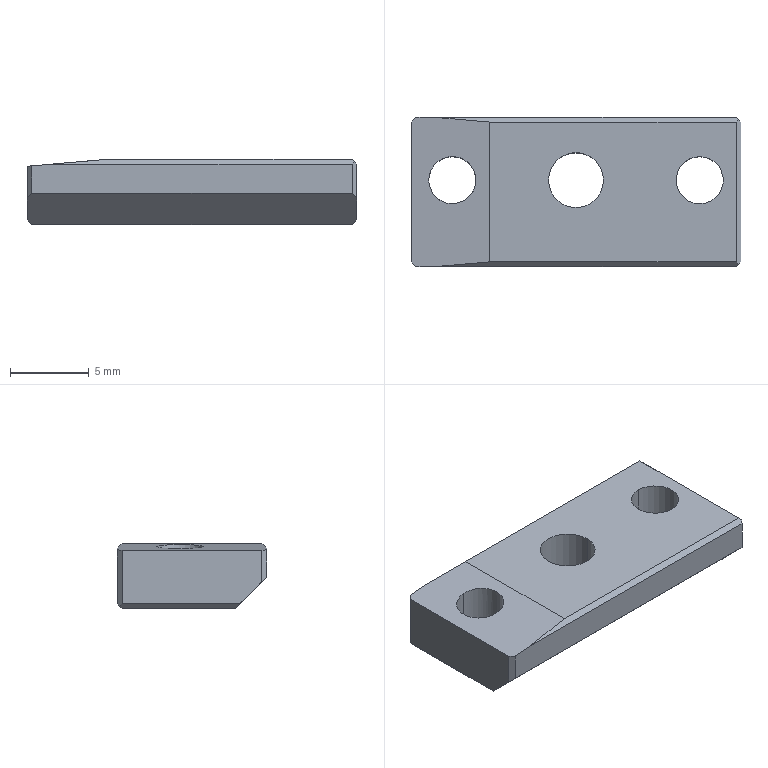Part | NX | 1 solid | 24 faces | box 21 x 9.5 x 4.15 mm | volume 674.351 mm3 | plane 18 | cylinder 6 | commonest cylinder face diameters 3 x4 3.5 x2
STEP:
#1=CARTESIAN_POINT('',(-137.,182.4,-96.5));
#2=VERTEX_POINT('',#1);
#3=CARTESIAN_POINT('',(-137.,173.5,-96.5));
#4=VERTEX_POINT('',#3);
#5=CARTESIAN_POINT('',(-137.,177.95,-96.5));
#6=DIRECTION('',(0.,-1.,0.));
#7=VECTOR('',#6,1000.);
#8=LINE('',#5,#7);
#9=EDGE_CURVE('',#2,#4,#8,.T.);
#10=ORIENTED_EDGE('',*,*,#9,.T.);
#11=CARTESIAN_POINT('',(-121.3,173.5,-96.5));
#12=VERTEX_POINT('',#11);
#13=CARTESIAN_POINT('',(-131.65,173.5,-96.5));
#14=DIRECTION('',(1.,0.,0.));
#15=VECTOR('',#14,1000.);
#16=LINE('',#13,#15);
#17=EDGE_CURVE('',#4,#12,#16,.T.);
#18=ORIENTED_EDGE('',*,*,#17,.T.);
#19=CARTESIAN_POINT('',(-121.3,182.4,-96.5));
#20=VERTEX_POINT('',#19);
#21=CARTESIAN_POINT('',(-121.3,177.95,-96.5));
#22=DIRECTION('',(0.,-1.,0.));
#23=VECTOR('',#22,1000.);
#24=LINE('',#21,#23);
#25=EDGE_CURVE('',#20,#12,#24,.T.);
#26=ORIENTED_EDGE('',*,*,#25,.F.);
#27=CARTESIAN_POINT('',(-131.65,182.4,-96.5));
#28=DIRECTION('',(-1.,0.,0.));
#29=VECTOR('',#28,1000.);
#30=LINE('',#27,#29);
#31=EDGE_CURVE('',#20,#2,#30,.T.);
#32=ORIENTED_EDGE('',*,*,#31,.T.);
#33=EDGE_LOOP('',(#10,#18,#26,#32));
#34=FACE_BOUND('',#33,.T.);
#35=CARTESIAN_POINT('',(-123.625,180.2,-96.5));
#36=VERTEX_POINT('',#35);
#37=CARTESIAN_POINT('',(-123.625,177.2,-96.5));
#38=VERTEX_POINT('',#37);
#39=CARTESIAN_POINT('',(-123.625,178.7,-96.5));
#40=DIRECTION('',(0.,0.,-1.));
#41=DIRECTION('',(0.,-1.,0.));
#42=AXIS2_PLACEMENT_3D('',#39,#40,#41);
#43=CIRCLE('',#42,1.5);
#44=EDGE_CURVE('',#36,#38,#43,.T.);
#45=ORIENTED_EDGE('',*,*,#44,.T.);
#46=CARTESIAN_POINT('',(-123.625,178.7,-96.5));
#47=DIRECTION('',(0.,0.,-1.));
#48=DIRECTION('',(0.,-1.,0.));
#49=AXIS2_PLACEMENT_3D('',#46,#47,#48);
#50=CIRCLE('',#49,1.5);
#51=EDGE_CURVE('',#38,#36,#50,.T.);
#52=ORIENTED_EDGE('',*,*,#51,.T.);
#53=EDGE_LOOP('',(#45,#52));
#54=FACE_BOUND('',#53,.T.);
#55=CARTESIAN_POINT('',(-129.75,178.7,-96.5));
#56=VERTEX_POINT('',#55);
#57=CARTESIAN_POINT('',(-133.25,178.7,-96.5));
#58=VERTEX_POINT('',#57);
#59=CARTESIAN_POINT('',(-131.5,178.7,-96.5));
#60=DIRECTION('',(0.,0.,-1.));
#61=DIRECTION('',(-1.,0.,0.));
#62=AXIS2_PLACEMENT_3D('',#59,#60,#61);
#63=CIRCLE('',#62,1.75);
#64=EDGE_CURVE('',#56,#58,#63,.T.);
#65=ORIENTED_EDGE('',*,*,#64,.T.);
#66=CARTESIAN_POINT('',(-131.5,178.7,-96.5));
#67=DIRECTION('',(0.,0.,-1.));
#68=DIRECTION('',(-1.,0.,0.));
#69=AXIS2_PLACEMENT_3D('',#66,#67,#68);
#70=CIRCLE('',#69,1.75);
#71=EDGE_CURVE('',#58,#56,#70,.T.);
#72=ORIENTED_EDGE('',*,*,#71,.T.);
#73=EDGE_LOOP('',(#65,#72));
#74=FACE_BOUND('',#73,.T.);
#75=CARTESIAN_POINT('',(-121.,182.7,-96.5));
#76=DIRECTION('',(0.,0.,1.));
#77=DIRECTION('',(1.,0.,0.));
#78=AXIS2_PLACEMENT_3D('',#75,#76,#77);
#79=PLANE('',#78);
#80=ADVANCED_FACE('',(#34,#54,#74),#79,.T.);
#81=CARTESIAN_POINT('',(-121.3,182.7,-96.8));
#82=VERTEX_POINT('',#81);
#83=CARTESIAN_POINT('',(-140.429,182.7,-96.8));
#84=VERTEX_POINT('',#83);
#85=CARTESIAN_POINT('',(-131.65,182.7,-96.8));
#86=DIRECTION('',(-1.,0.,0.));
#87=VECTOR('',#86,1000.);
#88=LINE('',#85,#87);
#89=EDGE_CURVE('',#82,#84,#88,.T.);
#90=ORIENTED_EDGE('',*,*,#89,.F.);
#91=CARTESIAN_POINT('',(-121.3,182.7,-100.35));
#92=VERTEX_POINT('',#91);
#93=CARTESIAN_POINT('',(-121.3,182.7,-98.575));
#94=DIRECTION('',(0.,0.,1.));
#95=VECTOR('',#94,1000.);
#96=LINE('',#93,#95);
#97=EDGE_CURVE('',#92,#82,#96,.T.);
#98=ORIENTED_EDGE('',*,*,#97,.F.);
#99=CARTESIAN_POINT('',(-141.7,182.7,-100.35));
#100=VERTEX_POINT('',#99);
#101=CARTESIAN_POINT('',(-131.5,182.7,-100.35));
#102=DIRECTION('',(-1.,0.,0.));
#103=VECTOR('',#102,1000.);
#104=LINE('',#101,#103);
#105=EDGE_CURVE('',#92,#100,#104,.T.);
#106=ORIENTED_EDGE('',*,*,#105,.T.);
#107=CARTESIAN_POINT('',(-141.7,182.7,-96.911));
#108=VERTEX_POINT('',#107);
#109=CARTESIAN_POINT('',(-141.7,182.7,-98.425));
#110=DIRECTION('',(0.,0.,1.));
#111=VECTOR('',#110,1000.);
#112=LINE('',#109,#111);
#113=EDGE_CURVE('',#100,#108,#112,.T.);
#114=ORIENTED_EDGE('',*,*,#113,.T.);
#115=CARTESIAN_POINT('',(-121.,182.7,-95.1));
#116=DIRECTION('',(-0.9962,0.,-0.08716));
#117=VECTOR('',#116,1000.);
#118=LINE('',#115,#117);
#119=EDGE_CURVE('',#84,#108,#118,.T.);
#120=ORIENTED_EDGE('',*,*,#119,.F.);
#121=EDGE_LOOP('',(#90,#98,#106,#114,#120));
#122=FACE_BOUND('',#121,.T.);
#123=CARTESIAN_POINT('',(-121.,182.7,-100.65));
#124=DIRECTION('',(0.,1.,0.));
#125=DIRECTION('',(1.,0.,0.));
#126=AXIS2_PLACEMENT_3D('',#123,#124,#125);
#127=PLANE('',#126);
#128=ADVANCED_FACE('',(#122),#127,.T.);
#129=CARTESIAN_POINT('',(-121.3,175.2,-100.65));
#130=VERTEX_POINT('',#129);
#131=CARTESIAN_POINT('',(-141.7,175.2,-100.65));
#132=VERTEX_POINT('',#131);
#133=CARTESIAN_POINT('',(-131.5,175.2,-100.65));
#134=DIRECTION('',(-1.,0.,0.));
#135=VECTOR('',#134,1000.);
#136=LINE('',#133,#135);
#137=EDGE_CURVE('',#130,#132,#136,.T.);
#138=ORIENTED_EDGE('',*,*,#137,.T.);
#139=CARTESIAN_POINT('',(-141.7,182.4,-100.65));
#140=VERTEX_POINT('',#139);
#141=CARTESIAN_POINT('',(-141.7,178.95,-100.65));
#142=DIRECTION('',(0.,1.,0.));
#143=VECTOR('',#142,1000.);
#144=LINE('',#141,#143);
#145=EDGE_CURVE('',#132,#140,#144,.T.);
#146=ORIENTED_EDGE('',*,*,#145,.T.);
#147=CARTESIAN_POINT('',(-121.3,182.4,-100.65));
#148=VERTEX_POINT('',#147);
#149=CARTESIAN_POINT('',(-131.5,182.4,-100.65));
#150=DIRECTION('',(-1.,0.,0.));
#151=VECTOR('',#150,1000.);
#152=LINE('',#149,#151);
#153=EDGE_CURVE('',#148,#140,#152,.T.);
#154=ORIENTED_EDGE('',*,*,#153,.F.);
#155=CARTESIAN_POINT('',(-121.3,178.95,-100.65));
#156=DIRECTION('',(0.,1.,0.));
#157=VECTOR('',#156,1000.);
#158=LINE('',#155,#157);
#159=EDGE_CURVE('',#130,#148,#158,.T.);
#160=ORIENTED_EDGE('',*,*,#159,.F.);
#161=EDGE_LOOP('',(#138,#146,#154,#160));
#162=FACE_BOUND('',#161,.T.);
#163=CARTESIAN_POINT('',(-129.75,178.7,-100.65));
#164=VERTEX_POINT('',#163);
#165=CARTESIAN_POINT('',(-133.25,178.7,-100.65));
#166=VERTEX_POINT('',#165);
#167=CARTESIAN_POINT('',(-131.5,178.7,-100.65));
#168=DIRECTION('',(0.,0.,-1.));
#169=DIRECTION('',(-1.,0.,0.));
#170=AXIS2_PLACEMENT_3D('',#167,#168,#169);
#171=CIRCLE('',#170,1.75);
#172=EDGE_CURVE('',#164,#166,#171,.T.);
#173=ORIENTED_EDGE('',*,*,#172,.F.);
#174=CARTESIAN_POINT('',(-131.5,178.7,-100.65));
#175=DIRECTION('',(0.,0.,-1.));
#176=DIRECTION('',(-1.,0.,0.));
#177=AXIS2_PLACEMENT_3D('',#174,#175,#176);
#178=CIRCLE('',#177,1.75);
#179=EDGE_CURVE('',#166,#164,#178,.T.);
#180=ORIENTED_EDGE('',*,*,#179,.F.);
#181=EDGE_LOOP('',(#173,#180));
#182=FACE_BOUND('',#181,.T.);
#183=CARTESIAN_POINT('',(-123.625,180.2,-100.65));
#184=VERTEX_POINT('',#183);
#185=CARTESIAN_POINT('',(-123.625,177.2,-100.65));
#186=VERTEX_POINT('',#185);
#187=CARTESIAN_POINT('',(-123.625,178.7,-100.65));
#188=DIRECTION('',(0.,0.,-1.));
#189=DIRECTION('',(0.,-1.,0.));
#190=AXIS2_PLACEMENT_3D('',#187,#188,#189);
#191=CIRCLE('',#190,1.5);
#192=EDGE_CURVE('',#184,#186,#191,.T.);
#193=ORIENTED_EDGE('',*,*,#192,.F.);
#194=CARTESIAN_POINT('',(-123.625,178.7,-100.65));
#195=DIRECTION('',(0.,0.,-1.));
#196=DIRECTION('',(0.,-1.,0.));
#197=AXIS2_PLACEMENT_3D('',#194,#195,#196);
#198=CIRCLE('',#197,1.5);
#199=EDGE_CURVE('',#186,#184,#198,.T.);
#200=ORIENTED_EDGE('',*,*,#199,.F.);
#201=EDGE_LOOP('',(#193,#200));
#202=FACE_BOUND('',#201,.T.);
#203=CARTESIAN_POINT('',(-139.375,180.2,-100.65));
#204=VERTEX_POINT('',#203);
#205=CARTESIAN_POINT('',(-139.375,177.2,-100.65));
#206=VERTEX_POINT('',#205);
#207=CARTESIAN_POINT('',(-139.375,178.7,-100.65));
#208=DIRECTION('',(0.,0.,-1.));
#209=DIRECTION('',(0.,-1.,0.));
#210=AXIS2_PLACEMENT_3D('',#207,#208,#209);
#211=CIRCLE('',#210,1.5);
#212=EDGE_CURVE('',#204,#206,#211,.T.);
#213=ORIENTED_EDGE('',*,*,#212,.F.);
#214=CARTESIAN_POINT('',(-139.375,178.7,-100.65));
#215=DIRECTION('',(0.,0.,-1.));
#216=DIRECTION('',(0.,-1.,0.));
#217=AXIS2_PLACEMENT_3D('',#214,#215,#216);
#218=CIRCLE('',#217,1.5);
#219=EDGE_CURVE('',#206,#204,#218,.T.);
#220=ORIENTED_EDGE('',*,*,#219,.F.);
#221=EDGE_LOOP('',(#213,#220));
#222=FACE_BOUND('',#221,.T.);
#223=CARTESIAN_POINT('',(-121.,173.2,-100.65));
#224=DIRECTION('',(0.,0.,-1.));
#225=DIRECTION('',(0.,-1.,0.));
#226=AXIS2_PLACEMENT_3D('',#223,#224,#225);
#227=PLANE('',#226);
#228=ADVANCED_FACE('',(#162,#182,#202,#222),#227,.T.);
#229=CARTESIAN_POINT('',(-141.7,173.2,-96.911));
#230=VERTEX_POINT('',#229);
#231=CARTESIAN_POINT('',(-141.7,173.2,-98.65));
#232=VERTEX_POINT('',#231);
#233=CARTESIAN_POINT('',(-141.7,173.2,-97.575));
#234=DIRECTION('',(0.,0.,-1.));
#235=VECTOR('',#234,1000.);
#236=LINE('',#233,#235);
#237=EDGE_CURVE('',#230,#232,#236,.T.);
#238=ORIENTED_EDGE('',*,*,#237,.T.);
#239=CARTESIAN_POINT('',(-121.3,173.2,-98.65));
#240=VERTEX_POINT('',#239);
#241=CARTESIAN_POINT('',(-131.5,173.2,-98.65));
#242=DIRECTION('',(-1.,0.,0.));
#243=VECTOR('',#242,1000.);
#244=LINE('',#241,#243);
#245=EDGE_CURVE('',#240,#232,#244,.T.);
#246=ORIENTED_EDGE('',*,*,#245,.F.);
#247=CARTESIAN_POINT('',(-121.3,173.2,-96.8));
#248=VERTEX_POINT('',#247);
#249=CARTESIAN_POINT('',(-121.3,173.2,-97.575));
#250=DIRECTION('',(0.,0.,-1.));
#251=VECTOR('',#250,1000.);
#252=LINE('',#249,#251);
#253=EDGE_CURVE('',#248,#240,#252,.T.);
#254=ORIENTED_EDGE('',*,*,#253,.F.);
#255=CARTESIAN_POINT('',(-140.429,173.2,-96.8));
#256=VERTEX_POINT('',#255);
#257=CARTESIAN_POINT('',(-131.65,173.2,-96.8));
#258=DIRECTION('',(1.,0.,0.));
#259=VECTOR('',#258,1000.);
#260=LINE('',#257,#259);
#261=EDGE_CURVE('',#256,#248,#260,.T.);
#262=ORIENTED_EDGE('',*,*,#261,.F.);
#263=CARTESIAN_POINT('',(-121.,173.2,-95.1));
#264=DIRECTION('',(0.9962,0.,0.08716));
#265=VECTOR('',#264,1000.);
#266=LINE('',#263,#265);
#267=EDGE_CURVE('',#230,#256,#266,.T.);
#268=ORIENTED_EDGE('',*,*,#267,.F.);
#269=EDGE_LOOP('',(#238,#246,#254,#262,#268));
#270=FACE_BOUND('',#269,.T.);
#271=CARTESIAN_POINT('',(-121.,173.2,-96.5));
#272=DIRECTION('',(0.,-1.,0.));
#273=DIRECTION('',(0.,0.,-1.));
#274=AXIS2_PLACEMENT_3D('',#271,#272,#273);
#275=PLANE('',#274);
#276=ADVANCED_FACE('',(#270),#275,.T.);
#277=ORIENTED_EDGE('',*,*,#137,.F.);
#278=CARTESIAN_POINT('',(-121.,174.9,-100.35));
#279=VERTEX_POINT('',#278);
#280=CARTESIAN_POINT('',(-106.733,160.633,-86.083));
#281=DIRECTION('',(-0.5774,0.5774,-0.5774));
#282=VECTOR('',#281,1000.);
#283=LINE('',#280,#282);
#284=EDGE_CURVE('',#279,#130,#283,.T.);
#285=ORIENTED_EDGE('',*,*,#284,.F.);
#286=CARTESIAN_POINT('',(-121.,173.5,-98.95));
#287=VERTEX_POINT('',#286);
#288=CARTESIAN_POINT('',(-121.,160.633,-86.083));
#289=DIRECTION('',(0.,-0.7071,0.7071));
#290=VECTOR('',#289,1000.);
#291=LINE('',#288,#290);
#292=EDGE_CURVE('',#279,#287,#291,.T.);
#293=ORIENTED_EDGE('',*,*,#292,.T.);
#294=CARTESIAN_POINT('',(-121.,173.5,-98.95));
#295=DIRECTION('',(0.5774,0.5774,-0.5774));
#296=VECTOR('',#295,1000.);
#297=LINE('',#294,#296);
#298=EDGE_CURVE('',#240,#287,#297,.T.);
#299=ORIENTED_EDGE('',*,*,#298,.F.);
#300=ORIENTED_EDGE('',*,*,#245,.T.);
#301=CARTESIAN_POINT('',(-142.,173.5,-98.95));
#302=VERTEX_POINT('',#301);
#303=CARTESIAN_POINT('',(-121.,152.5,-77.95));
#304=DIRECTION('',(-0.5774,0.5774,-0.5774));
#305=VECTOR('',#304,1000.);
#306=LINE('',#303,#305);
#307=EDGE_CURVE('',#232,#302,#306,.T.);
#308=ORIENTED_EDGE('',*,*,#307,.T.);
#309=CARTESIAN_POINT('',(-142.,174.9,-100.35));
#310=VERTEX_POINT('',#309);
#311=CARTESIAN_POINT('',(-142.,160.633,-86.083));
#312=DIRECTION('',(0.,-0.7071,0.7071));
#313=VECTOR('',#312,1000.);
#314=LINE('',#311,#313);
#315=EDGE_CURVE('',#310,#302,#314,.T.);
#316=ORIENTED_EDGE('',*,*,#315,.F.);
#317=CARTESIAN_POINT('',(-121.,195.9,-121.35));
#318=DIRECTION('',(0.5774,0.5774,-0.5774));
#319=VECTOR('',#318,1000.);
#320=LINE('',#317,#319);
#321=EDGE_CURVE('',#310,#132,#320,.T.);
#322=ORIENTED_EDGE('',*,*,#321,.T.);
#323=EDGE_LOOP('',(#277,#285,#293,#299,#300,#308,#316,#322));
#324=FACE_BOUND('',#323,.T.);
#325=CARTESIAN_POINT('',(-131.5,174.2,-99.65));
#326=DIRECTION('',(0.,-0.7071,-0.7071));
#327=DIRECTION('',(0.,0.7071,-0.7071));
#328=AXIS2_PLACEMENT_3D('',#325,#326,#327);
#329=PLANE('',#328);
#330=ADVANCED_FACE('',(#324),#329,.T.);
#331=ORIENTED_EDGE('',*,*,#44,.F.);
#332=CARTESIAN_POINT('',(-123.625,180.2,-96.085));
#333=DIRECTION('',(0.,0.,-1.));
#334=VECTOR('',#333,1000.);
#335=LINE('',#332,#334);
#336=EDGE_CURVE('',#184,#36,#335,.F.);
#337=ORIENTED_EDGE('',*,*,#336,.F.);
#338=ORIENTED_EDGE('',*,*,#192,.T.);
#339=CARTESIAN_POINT('',(-123.625,177.2,-96.085));
#340=DIRECTION('',(0.,0.,-1.));
#341=VECTOR('',#340,1000.);
#342=LINE('',#339,#341);
#343=EDGE_CURVE('',#186,#38,#342,.F.);
#344=ORIENTED_EDGE('',*,*,#343,.T.);
#345=EDGE_LOOP('',(#331,#337,#338,#344));
#346=FACE_BOUND('',#345,.T.);
#347=CARTESIAN_POINT('',(-123.625,178.7,-96.085));
#348=DIRECTION('',(0.,0.,-1.));
#349=DIRECTION('',(0.,-1.,0.));
#350=AXIS2_PLACEMENT_3D('',#347,#348,#349);
#351=CYLINDRICAL_SURFACE('',#350,1.5);
#352=ADVANCED_FACE('',(#346),#351,.F.);
#353=ORIENTED_EDGE('',*,*,#9,.F.);
#354=CARTESIAN_POINT('',(-121.,181.,-95.1));
#355=DIRECTION('',(-0.9924,0.08683,-0.08683));
#356=VECTOR('',#355,1000.);
#357=LINE('',#354,#356);
#358=EDGE_CURVE('',#2,#84,#357,.T.);
#359=ORIENTED_EDGE('',*,*,#358,.T.);
#360=ORIENTED_EDGE('',*,*,#119,.T.);
#361=CARTESIAN_POINT('',(-142.,182.4,-96.937));
#362=VERTEX_POINT('',#361);
#363=CARTESIAN_POINT('',(-121.,203.4,-95.1));
#364=DIRECTION('',(0.7058,0.7058,0.06175));
#365=VECTOR('',#364,1000.);
#366=LINE('',#363,#365);
#367=EDGE_CURVE('',#362,#108,#366,.T.);
#368=ORIENTED_EDGE('',*,*,#367,.F.);
#369=CARTESIAN_POINT('',(-142.,173.5,-96.937));
#370=VERTEX_POINT('',#369);
#371=CARTESIAN_POINT('',(-142.,177.95,-96.937));
#372=DIRECTION('',(0.,-1.,0.));
#373=VECTOR('',#372,1000.);
#374=LINE('',#371,#373);
#375=EDGE_CURVE('',#362,#370,#374,.T.);
#376=ORIENTED_EDGE('',*,*,#375,.T.);
#377=CARTESIAN_POINT('',(-121.,152.5,-95.1));
#378=DIRECTION('',(-0.7058,0.7058,-0.06175));
#379=VECTOR('',#378,1000.);
#380=LINE('',#377,#379);
#381=EDGE_CURVE('',#230,#370,#380,.T.);
#382=ORIENTED_EDGE('',*,*,#381,.F.);
#383=ORIENTED_EDGE('',*,*,#267,.T.);
#384=CARTESIAN_POINT('',(-121.,174.9,-95.1));
#385=DIRECTION('',(0.9924,0.08683,0.08683));
#386=VECTOR('',#385,1000.);
#387=LINE('',#384,#386);
#388=EDGE_CURVE('',#256,#4,#387,.T.);
#389=ORIENTED_EDGE('',*,*,#388,.T.);
#390=EDGE_LOOP('',(#353,#359,#360,#368,#376,#382,#383,#389));
#391=FACE_BOUND('',#390,.T.);
#392=CARTESIAN_POINT('',(-139.375,180.2,-96.708));
#393=VERTEX_POINT('',#392);
#394=CARTESIAN_POINT('',(-139.375,177.2,-96.708));
#395=VERTEX_POINT('',#394);
#396=CARTESIAN_POINT('',(-139.375,180.2,-96.708));
#397=CARTESIAN_POINT('',(-142.375,180.2,-96.97));
#398=CARTESIAN_POINT('',(-142.375,177.2,-96.97));
#399=CARTESIAN_POINT('',(-139.375,177.2,-96.708));
#400=(BOUNDED_CURVE()B_SPLINE_CURVE(3,(#396,#397,#398,#399),.UNSPECIFIED.,.F.,.F.)B_SPLINE_CURVE_WITH_KNOTS((4,4),(4.712,7.854),.UNSPECIFIED.)CURVE()GEOMETRIC_REPRESENTATION_ITEM()RATIONAL_B_SPLINE_CURVE((1.,0.3333,0.3333,1.))REPRESENTATION_ITEM(''));
#401=EDGE_CURVE('',#393,#395,#400,.T.);
#402=ORIENTED_EDGE('',*,*,#401,.F.);
#403=CARTESIAN_POINT('',(-139.375,177.2,-96.708));
#404=CARTESIAN_POINT('',(-136.375,177.2,-96.445));
#405=CARTESIAN_POINT('',(-136.375,180.2,-96.445));
#406=CARTESIAN_POINT('',(-139.375,180.2,-96.708));
#407=(BOUNDED_CURVE()B_SPLINE_CURVE(3,(#403,#404,#405,#406),.UNSPECIFIED.,.F.,.F.)B_SPLINE_CURVE_WITH_KNOTS((4,4),(1.571,4.712),.UNSPECIFIED.)CURVE()GEOMETRIC_REPRESENTATION_ITEM()RATIONAL_B_SPLINE_CURVE((1.,0.3333,0.3333,1.))REPRESENTATION_ITEM(''));
#408=EDGE_CURVE('',#395,#393,#407,.T.);
#409=ORIENTED_EDGE('',*,*,#408,.F.);
#410=EDGE_LOOP('',(#402,#409));
#411=FACE_BOUND('',#410,.T.);
#412=CARTESIAN_POINT('',(-139.5,177.95,-96.719));
#413=DIRECTION('',(-0.08716,0.,0.9962));
#414=DIRECTION('',(0.,1.,0.));
#415=AXIS2_PLACEMENT_3D('',#412,#413,#414);
#416=PLANE('',#415);
#417=ADVANCED_FACE('',(#391,#411),#416,.T.);
#418=ORIENTED_EDGE('',*,*,#64,.F.);
#419=CARTESIAN_POINT('',(-129.75,178.7,-96.085));
#420=DIRECTION('',(0.,0.,-1.));
#421=VECTOR('',#420,1000.);
#422=LINE('',#419,#421);
#423=EDGE_CURVE('',#164,#56,#422,.F.);
#424=ORIENTED_EDGE('',*,*,#423,.F.);
#425=ORIENTED_EDGE('',*,*,#172,.T.);
#426=CARTESIAN_POINT('',(-133.25,178.7,-96.085));
#427=DIRECTION('',(0.,0.,-1.));
#428=VECTOR('',#427,1000.);
#429=LINE('',#426,#428);
#430=EDGE_CURVE('',#166,#58,#429,.F.);
#431=ORIENTED_EDGE('',*,*,#430,.T.);
#432=EDGE_LOOP('',(#418,#424,#425,#431));
#433=FACE_BOUND('',#432,.T.);
#434=CARTESIAN_POINT('',(-131.5,178.7,-96.085));
#435=DIRECTION('',(0.,0.,-1.));
#436=DIRECTION('',(-1.,0.,0.));
#437=AXIS2_PLACEMENT_3D('',#434,#435,#436);
#438=CYLINDRICAL_SURFACE('',#437,1.75);
#439=ADVANCED_FACE('',(#433),#438,.F.);
#440=ORIENTED_EDGE('',*,*,#105,.F.);
#441=CARTESIAN_POINT('',(-121.15,182.55,-100.5));
#442=VERTEX_POINT('',#441);
#443=CARTESIAN_POINT('',(-135.567,196.967,-86.083));
#444=DIRECTION('',(0.5774,-0.5774,-0.5774));
#445=VECTOR('',#444,1000.);
#446=LINE('',#443,#445);
#447=EDGE_CURVE('',#92,#442,#446,.T.);
#448=ORIENTED_EDGE('',*,*,#447,.T.);
#449=CARTESIAN_POINT('',(-106.733,196.967,-86.083));
#450=DIRECTION('',(0.5774,0.5774,0.5774));
#451=VECTOR('',#450,1000.);
#452=LINE('',#449,#451);
#453=EDGE_CURVE('',#148,#442,#452,.T.);
#454=ORIENTED_EDGE('',*,*,#453,.F.);
#455=ORIENTED_EDGE('',*,*,#153,.T.);
#456=CARTESIAN_POINT('',(-141.85,182.55,-100.5));
#457=VERTEX_POINT('',#456);
#458=CARTESIAN_POINT('',(-121.,161.7,-121.35));
#459=DIRECTION('',(0.5774,-0.5774,-0.5774));
#460=VECTOR('',#459,1000.);
#461=LINE('',#458,#460);
#462=EDGE_CURVE('',#457,#140,#461,.T.);
#463=ORIENTED_EDGE('',*,*,#462,.F.);
#464=CARTESIAN_POINT('',(-121.,203.4,-79.65));
#465=DIRECTION('',(0.5774,0.5774,0.5774));
#466=VECTOR('',#465,1000.);
#467=LINE('',#464,#466);
#468=EDGE_CURVE('',#457,#100,#467,.T.);
#469=ORIENTED_EDGE('',*,*,#468,.T.);
#470=EDGE_LOOP('',(#440,#448,#454,#455,#463,#469));
#471=FACE_BOUND('',#470,.T.);
#472=CARTESIAN_POINT('',(-131.5,182.55,-100.5));
#473=DIRECTION('',(0.,0.7071,-0.7071));
#474=DIRECTION('',(-1.,0.,0.));
#475=AXIS2_PLACEMENT_3D('',#472,#473,#474);
#476=PLANE('',#475);
#477=ADVANCED_FACE('',(#471),#476,.T.);
#478=ORIENTED_EDGE('',*,*,#17,.F.);
#479=ORIENTED_EDGE('',*,*,#388,.F.);
#480=ORIENTED_EDGE('',*,*,#261,.T.);
#481=CARTESIAN_POINT('',(-121.15,173.35,-96.65));
#482=VERTEX_POINT('',#481);
#483=CARTESIAN_POINT('',(-121.,173.5,-96.5));
#484=DIRECTION('',(0.5774,0.5774,0.5774));
#485=VECTOR('',#484,1000.);
#486=LINE('',#483,#485);
#487=EDGE_CURVE('',#248,#482,#486,.T.);
#488=ORIENTED_EDGE('',*,*,#487,.T.);
#489=CARTESIAN_POINT('',(-131.717,183.917,-86.083));
#490=DIRECTION('',(-0.5774,0.5774,0.5774));
#491=VECTOR('',#490,1000.);
#492=LINE('',#489,#491);
#493=EDGE_CURVE('',#482,#12,#492,.T.);
#494=ORIENTED_EDGE('',*,*,#493,.T.);
#495=EDGE_LOOP('',(#478,#479,#480,#488,#494));
#496=FACE_BOUND('',#495,.T.);
#497=CARTESIAN_POINT('',(-131.65,173.35,-96.65));
#498=DIRECTION('',(0.,-0.7071,0.7071));
#499=DIRECTION('',(-1.,0.,0.));
#500=AXIS2_PLACEMENT_3D('',#497,#498,#499);
#501=PLANE('',#500);
#502=ADVANCED_FACE('',(#496),#501,.T.);
#503=ORIENTED_EDGE('',*,*,#31,.F.);
#504=CARTESIAN_POINT('',(-121.15,182.55,-96.65));
#505=VERTEX_POINT('',#504);
#506=CARTESIAN_POINT('',(-131.717,171.983,-86.083));
#507=DIRECTION('',(0.5774,0.5774,-0.5774));
#508=VECTOR('',#507,1000.);
#509=LINE('',#506,#508);
#510=EDGE_CURVE('',#20,#505,#509,.T.);
#511=ORIENTED_EDGE('',*,*,#510,.T.);
#512=CARTESIAN_POINT('',(-110.583,171.983,-86.083));
#513=DIRECTION('',(-0.5774,0.5774,-0.5774));
#514=VECTOR('',#513,1000.);
#515=LINE('',#512,#514);
#516=EDGE_CURVE('',#505,#82,#515,.T.);
#517=ORIENTED_EDGE('',*,*,#516,.T.);
#518=ORIENTED_EDGE('',*,*,#89,.T.);
#519=ORIENTED_EDGE('',*,*,#358,.F.);
#520=EDGE_LOOP('',(#503,#511,#517,#518,#519));
#521=FACE_BOUND('',#520,.T.);
#522=CARTESIAN_POINT('',(-131.65,182.55,-96.65));
#523=DIRECTION('',(0.,0.7071,0.7071));
#524=DIRECTION('',(1.,0.,0.));
#525=AXIS2_PLACEMENT_3D('',#522,#523,#524);
#526=PLANE('',#525);
#527=ADVANCED_FACE('',(#521),#526,.T.);
#528=ORIENTED_EDGE('',*,*,#401,.T.);
#529=CARTESIAN_POINT('',(-139.375,177.2,-96.085));
#530=DIRECTION('',(0.,0.,-1.));
#531=VECTOR('',#530,1000.);
#532=LINE('',#529,#531);
#533=EDGE_CURVE('',#206,#395,#532,.F.);
#534=ORIENTED_EDGE('',*,*,#533,.F.);
#535=ORIENTED_EDGE('',*,*,#219,.T.);
#536=CARTESIAN_POINT('',(-139.375,180.2,-96.085));
#537=DIRECTION('',(0.,0.,-1.));
#538=VECTOR('',#537,1000.);
#539=LINE('',#536,#538);
#540=EDGE_CURVE('',#204,#393,#539,.F.);
#541=ORIENTED_EDGE('',*,*,#540,.T.);
#542=EDGE_LOOP('',(#528,#534,#535,#541));
#543=FACE_BOUND('',#542,.T.);
#544=CARTESIAN_POINT('',(-139.375,178.7,-96.085));
#545=DIRECTION('',(0.,0.,-1.));
#546=DIRECTION('',(0.,-1.,0.));
#547=AXIS2_PLACEMENT_3D('',#544,#545,#546);
#548=CYLINDRICAL_SURFACE('',#547,1.5);
#549=ADVANCED_FACE('',(#543),#548,.F.);
#550=ORIENTED_EDGE('',*,*,#430,.F.);
#551=ORIENTED_EDGE('',*,*,#179,.T.);
#552=ORIENTED_EDGE('',*,*,#423,.T.);
#553=ORIENTED_EDGE('',*,*,#71,.F.);
#554=EDGE_LOOP('',(#550,#551,#552,#553));
#555=FACE_BOUND('',#554,.T.);
#556=CARTESIAN_POINT('',(-131.5,178.7,-96.085));
#557=DIRECTION('',(0.,0.,-1.));
#558=DIRECTION('',(-1.,0.,0.));
#559=AXIS2_PLACEMENT_3D('',#556,#557,#558);
#560=CYLINDRICAL_SURFACE('',#559,1.75);
#561=ADVANCED_FACE('',(#555),#560,.F.);
#562=ORIENTED_EDGE('',*,*,#212,.T.);
#563=ORIENTED_EDGE('',*,*,#533,.T.);
#564=ORIENTED_EDGE('',*,*,#408,.T.);
#565=ORIENTED_EDGE('',*,*,#540,.F.);
#566=EDGE_LOOP('',(#562,#563,#564,#565));
#567=FACE_BOUND('',#566,.T.);
#568=CARTESIAN_POINT('',(-139.375,178.7,-96.085));
#569=DIRECTION('',(0.,0.,-1.));
#570=DIRECTION('',(0.,-1.,0.));
#571=AXIS2_PLACEMENT_3D('',#568,#569,#570);
#572=CYLINDRICAL_SURFACE('',#571,1.5);
#573=ADVANCED_FACE('',(#567),#572,.F.);
#574=ORIENTED_EDGE('',*,*,#343,.F.);
#575=ORIENTED_EDGE('',*,*,#199,.T.);
#576=ORIENTED_EDGE('',*,*,#336,.T.);
#577=ORIENTED_EDGE('',*,*,#51,.F.);
#578=EDGE_LOOP('',(#574,#575,#576,#577));
#579=FACE_BOUND('',#578,.T.);
#580=CARTESIAN_POINT('',(-123.625,178.7,-96.085));
#581=DIRECTION('',(0.,0.,-1.));
#582=DIRECTION('',(0.,-1.,0.));
#583=AXIS2_PLACEMENT_3D('',#580,#581,#582);
#584=CYLINDRICAL_SURFACE('',#583,1.5);
#585=ADVANCED_FACE('',(#579),#584,.F.);
#586=CARTESIAN_POINT('',(-142.,182.4,-100.35));
#587=VERTEX_POINT('',#586);
#588=CARTESIAN_POINT('',(-142.,182.4,-98.425));
#589=DIRECTION('',(0.,0.,1.));
#590=VECTOR('',#589,1000.);
#591=LINE('',#588,#590);
#592=EDGE_CURVE('',#587,#362,#591,.T.);
#593=ORIENTED_EDGE('',*,*,#592,.F.);
#594=CARTESIAN_POINT('',(-142.,178.95,-100.35));
#595=DIRECTION('',(0.,1.,0.));
#596=VECTOR('',#595,1000.);
#597=LINE('',#594,#596);
#598=EDGE_CURVE('',#310,#587,#597,.T.);
#599=ORIENTED_EDGE('',*,*,#598,.F.);
#600=ORIENTED_EDGE('',*,*,#315,.T.);
#601=CARTESIAN_POINT('',(-142.,173.5,-97.575));
#602=DIRECTION('',(0.,0.,-1.));
#603=VECTOR('',#602,1000.);
#604=LINE('',#601,#603);
#605=EDGE_CURVE('',#370,#302,#604,.T.);
#606=ORIENTED_EDGE('',*,*,#605,.F.);
#607=ORIENTED_EDGE('',*,*,#375,.F.);
#608=EDGE_LOOP('',(#593,#599,#600,#606,#607));
#609=FACE_BOUND('',#608,.T.);
#610=CARTESIAN_POINT('',(-142.,177.442,-86.083));
#611=DIRECTION('',(1.,0.,0.));
#612=DIRECTION('',(0.,1.,0.));
#613=AXIS2_PLACEMENT_3D('',#610,#611,#612);
#614=PLANE('',#613);
#615=ADVANCED_FACE('',(#609),#614,.F.);
#616=ORIENTED_EDGE('',*,*,#598,.T.);
#617=CARTESIAN_POINT('',(-121.,203.4,-121.35));
#618=DIRECTION('',(-0.5774,-0.5774,0.5774));
#619=VECTOR('',#618,1000.);
#620=LINE('',#617,#619);
#621=EDGE_CURVE('',#457,#587,#620,.T.);
#622=ORIENTED_EDGE('',*,*,#621,.F.);
#623=ORIENTED_EDGE('',*,*,#462,.T.);
#624=ORIENTED_EDGE('',*,*,#145,.F.);
#625=ORIENTED_EDGE('',*,*,#321,.F.);
#626=EDGE_LOOP('',(#616,#622,#623,#624,#625));
#627=FACE_BOUND('',#626,.T.);
#628=CARTESIAN_POINT('',(-141.85,178.95,-100.5));
#629=DIRECTION('',(0.7071,0.,0.7071));
#630=DIRECTION('',(0.,-1.,0.));
#631=AXIS2_PLACEMENT_3D('',#628,#629,#630);
#632=PLANE('',#631);
#633=ADVANCED_FACE('',(#627),#632,.F.);
#634=ORIENTED_EDGE('',*,*,#605,.T.);
#635=ORIENTED_EDGE('',*,*,#307,.F.);
#636=ORIENTED_EDGE('',*,*,#237,.F.);
#637=ORIENTED_EDGE('',*,*,#381,.T.);
#638=EDGE_LOOP('',(#634,#635,#636,#637));
#639=FACE_BOUND('',#638,.T.);
#640=CARTESIAN_POINT('',(-141.85,173.35,-97.575));
#641=DIRECTION('',(0.7071,0.7071,0.));
#642=DIRECTION('',(0.,0.,-1.));
#643=AXIS2_PLACEMENT_3D('',#640,#641,#642);
#644=PLANE('',#643);
#645=ADVANCED_FACE('',(#639),#644,.F.);
#646=ORIENTED_EDGE('',*,*,#592,.T.);
#647=ORIENTED_EDGE('',*,*,#367,.T.);
#648=ORIENTED_EDGE('',*,*,#113,.F.);
#649=ORIENTED_EDGE('',*,*,#468,.F.);
#650=ORIENTED_EDGE('',*,*,#621,.T.);
#651=EDGE_LOOP('',(#646,#647,#648,#649,#650));
#652=FACE_BOUND('',#651,.T.);
#653=CARTESIAN_POINT('',(-141.85,182.55,-98.425));
#654=DIRECTION('',(0.7071,-0.7071,0.));
#655=DIRECTION('',(0.,0.,-1.));
#656=AXIS2_PLACEMENT_3D('',#653,#654,#655);
#657=PLANE('',#656);
#658=ADVANCED_FACE('',(#652),#657,.F.);
#659=CARTESIAN_POINT('',(-121.,173.5,-96.8));
#660=VERTEX_POINT('',#659);
#661=CARTESIAN_POINT('',(-121.,173.5,-97.575));
#662=DIRECTION('',(0.,0.,-1.));
#663=VECTOR('',#662,1000.);
#664=LINE('',#661,#663);
#665=EDGE_CURVE('',#660,#287,#664,.T.);
#666=ORIENTED_EDGE('',*,*,#665,.T.);
#667=ORIENTED_EDGE('',*,*,#292,.F.);
#668=CARTESIAN_POINT('',(-121.,182.4,-100.35));
#669=VERTEX_POINT('',#668);
#670=CARTESIAN_POINT('',(-121.,178.95,-100.35));
#671=DIRECTION('',(0.,1.,0.));
#672=VECTOR('',#671,1000.);
#673=LINE('',#670,#672);
#674=EDGE_CURVE('',#279,#669,#673,.T.);
#675=ORIENTED_EDGE('',*,*,#674,.T.);
#676=CARTESIAN_POINT('',(-121.,182.4,-96.8));
#677=VERTEX_POINT('',#676);
#678=CARTESIAN_POINT('',(-121.,182.4,-98.575));
#679=DIRECTION('',(0.,0.,1.));
#680=VECTOR('',#679,1000.);
#681=LINE('',#678,#680);
#682=EDGE_CURVE('',#669,#677,#681,.T.);
#683=ORIENTED_EDGE('',*,*,#682,.T.);
#684=CARTESIAN_POINT('',(-121.,177.95,-96.8));
#685=DIRECTION('',(0.,-1.,0.));
#686=VECTOR('',#685,1000.);
#687=LINE('',#684,#686);
#688=EDGE_CURVE('',#677,#660,#687,.T.);
#689=ORIENTED_EDGE('',*,*,#688,.T.);
#690=EDGE_LOOP('',(#666,#667,#675,#683,#689));
#691=FACE_BOUND('',#690,.T.);
#692=CARTESIAN_POINT('',(-121.,177.442,-86.083));
#693=DIRECTION('',(1.,0.,0.));
#694=DIRECTION('',(0.,1.,0.));
#695=AXIS2_PLACEMENT_3D('',#692,#693,#694);
#696=PLANE('',#695);
#697=ADVANCED_FACE('',(#691),#696,.T.);
#698=ORIENTED_EDGE('',*,*,#674,.F.);
#699=ORIENTED_EDGE('',*,*,#284,.T.);
#700=ORIENTED_EDGE('',*,*,#159,.T.);
#701=ORIENTED_EDGE('',*,*,#453,.T.);
#702=CARTESIAN_POINT('',(-116.042,177.442,-95.392));
#703=DIRECTION('',(0.5774,-0.5774,0.5774));
#704=VECTOR('',#703,1000.);
#705=LINE('',#702,#704);
#706=EDGE_CURVE('',#442,#669,#705,.T.);
#707=ORIENTED_EDGE('',*,*,#706,.T.);
#708=EDGE_LOOP('',(#698,#699,#700,#701,#707));
#709=FACE_BOUND('',#708,.T.);
#710=CARTESIAN_POINT('',(-121.15,178.95,-100.5));
#711=DIRECTION('',(0.7071,0.,-0.7071));
#712=DIRECTION('',(0.,-1.,0.));
#713=AXIS2_PLACEMENT_3D('',#710,#711,#712);
#714=PLANE('',#713);
#715=ADVANCED_FACE('',(#709),#714,.T.);
#716=ORIENTED_EDGE('',*,*,#682,.F.);
#717=ORIENTED_EDGE('',*,*,#706,.F.);
#718=ORIENTED_EDGE('',*,*,#447,.F.);
#719=ORIENTED_EDGE('',*,*,#97,.T.);
#720=ORIENTED_EDGE('',*,*,#516,.F.);
#721=CARTESIAN_POINT('',(-116.042,177.442,-101.758));
#722=DIRECTION('',(0.5774,-0.5774,-0.5774));
#723=VECTOR('',#722,1000.);
#724=LINE('',#721,#723);
#725=EDGE_CURVE('',#505,#677,#724,.T.);
#726=ORIENTED_EDGE('',*,*,#725,.T.);
#727=EDGE_LOOP('',(#716,#717,#718,#719,#720,#726));
#728=FACE_BOUND('',#727,.T.);
#729=CARTESIAN_POINT('',(-121.15,182.55,-98.575));
#730=DIRECTION('',(0.7071,0.7071,0.));
#731=DIRECTION('',(0.,0.,-1.));
#732=AXIS2_PLACEMENT_3D('',#729,#730,#731);
#733=PLANE('',#732);
#734=ADVANCED_FACE('',(#728),#733,.T.);
#735=ORIENTED_EDGE('',*,*,#688,.F.);
#736=ORIENTED_EDGE('',*,*,#725,.F.);
#737=ORIENTED_EDGE('',*,*,#510,.F.);
#738=ORIENTED_EDGE('',*,*,#25,.T.);
#739=ORIENTED_EDGE('',*,*,#493,.F.);
#740=CARTESIAN_POINT('',(-131.717,162.783,-86.083));
#741=DIRECTION('',(0.5774,0.5774,-0.5774));
#742=VECTOR('',#741,1000.);
#743=LINE('',#740,#742);
#744=EDGE_CURVE('',#482,#660,#743,.T.);
#745=ORIENTED_EDGE('',*,*,#744,.T.);
#746=EDGE_LOOP('',(#735,#736,#737,#738,#739,#745));
#747=FACE_BOUND('',#746,.T.);
#748=CARTESIAN_POINT('',(-121.15,177.95,-96.65));
#749=DIRECTION('',(0.7071,0.,0.7071));
#750=DIRECTION('',(0.,-1.,0.));
#751=AXIS2_PLACEMENT_3D('',#748,#749,#750);
#752=PLANE('',#751);
#753=ADVANCED_FACE('',(#747),#752,.T.);
#754=ORIENTED_EDGE('',*,*,#665,.F.);
#755=ORIENTED_EDGE('',*,*,#744,.F.);
#756=ORIENTED_EDGE('',*,*,#487,.F.);
#757=ORIENTED_EDGE('',*,*,#253,.T.);
#758=ORIENTED_EDGE('',*,*,#298,.T.);
#759=EDGE_LOOP('',(#754,#755,#756,#757,#758));
#760=FACE_BOUND('',#759,.T.);
#761=CARTESIAN_POINT('',(-121.15,173.35,-97.575));
#762=DIRECTION('',(0.7071,-0.7071,0.));
#763=DIRECTION('',(0.,0.,-1.));
#764=AXIS2_PLACEMENT_3D('',#761,#762,#763);
#765=PLANE('',#764);
#766=ADVANCED_FACE('',(#760),#765,.T.);
#767=CLOSED_SHELL('',(#80,#128,#228,#276,#330,#352,#417,#439,#477,#502,#527,#549,#561,#573,#585,#615,#633,#645,#658,#697,#715,#734,#753,#766));
#768=MANIFOLD_SOLID_BREP('',#767);
#769=(LENGTH_UNIT()NAMED_UNIT(*)SI_UNIT(.MILLI.,.METRE.));
#770=UNCERTAINTY_MEASURE_WITH_UNIT(LENGTH_MEASURE(0.00001),#769,'','');
#771=(NAMED_UNIT(*)PLANE_ANGLE_UNIT()SI_UNIT($,.RADIAN.));
#772=(NAMED_UNIT(*)SI_UNIT($,.STERADIAN.)SOLID_ANGLE_UNIT());
#773=(GEOMETRIC_REPRESENTATION_CONTEXT(3)GLOBAL_UNCERTAINTY_ASSIGNED_CONTEXT((#770))GLOBAL_UNIT_ASSIGNED_CONTEXT((#769,#771,#772))REPRESENTATION_CONTEXT('',''));
#774=ADVANCED_BREP_SHAPE_REPRESENTATION('',(#768),#773);